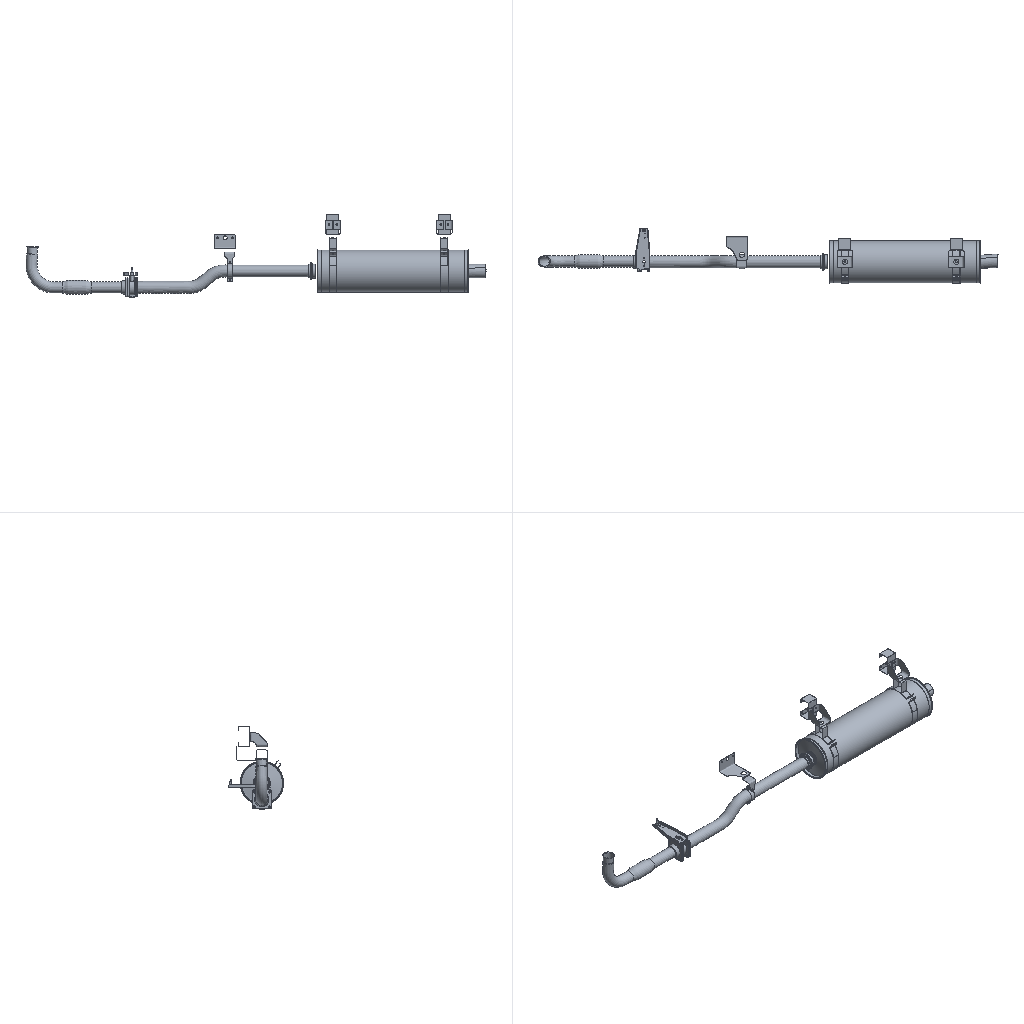Simulation study | nastran
Set-up summary:
category,name,step,type,value,unit,region
solver,nx_nastran
units,not stated in the deck,,not stated
analysis,deck,,modal,modal
analysis,solution,,SOL,103
load_step,SUBCASE 1,1,SUBCASE,SPC=None LOAD=None
mesh,nodes,,,119114
mesh,elements,,,239207
element_type,CQUAD4,,shell,54848
element_type,CTETRA,,solid,184005
element_type,CTRIA3,,shell,354
load,load commands in deck,,count,0
bc,support commands in deck,,count,0
check,setup vs results,,match,"every grid point's frame and coordinates and every element id; grid points of CQUAD4, CTETRA, CTRIA3 elements"
Nastran input file, long lists of numbers shortened:
$$------------------------------------------------------------------------------$
$$                                                                              $
$$ NASTRAN Input Deck Generated by HyperMesh Version  :10.0buil                 $
$$ Generated using HyperMesh-Nastran Template Version : 10.0build60
$$                                                                              $
$$   Template:  general                                                         $
$$                                                                              $
$$------------------------------------------------------------------------------$
$$------------------------------------------------------------------------------$
$$                      Executive Control Cards                                 $
$$------------------------------------------------------------------------------$
SOL 103
CEND
$$------------------------------------------------------------------------------$
$$                      Case Control Cards                                      $
$$------------------------------------------------------------------------------$
  DISPLACEMENT = ALL
$
$HMNAME LOADSTEP               1"modal"
SUBCASE       1
  LABEL= modal
  METHOD(STRUCTURE) =        1
$$------------------------------------------------------------------------------$
$$                      Bulk Data Cards                                         $
$$------------------------------------------------------------------------------$
BEGIN BULK
PARAM,POST,-1
$$
$$  GRID Data
$$
GRID          15        651.7036269.0462-556.3
GRID         158        651.0115268.8809-557.749
$ (119112 more lines like these left out)
$$
$$  SPOINT Data
$$
$$
$$------------------------------------------------------------------------------$
$$             Group Definitions                                                $
$$------------------------------------------------------------------------------$
$
$ RBE2 Elements - Single dependent node
$
RBE2        6841    4629  123456    3564
RBE2        6840    4628  123456    3563
$ (313 more lines like these left out)
$
$HMMOVE        8
$           6841    6840    6839    6838    6837    6836    6835    6834    6833
$           6832    6831    6830    6829    6828    6827    6826    6825    6824
$           6823    6822    6821    6820    6819    6818    6817    6816    6815
$           6814    6813    6812    6811    6810    6809    6808    6807    6806
$           6805    6804    6803    6802    6801    6800    6799    6798    6797
$           6796    6795    6794  648943THRU      648995  648997THRU      649001
$         649004THRU      649010  649012  649014  649016THRU      649020  649022
$       THRU      649024  649026THRU      649028  649033THRU      649035  649037
$         649039THRU      649040  649042THRU      649048  649050THRU      649053
$         649055THRU      649056  649058THRU      649059  649061THRU      649063
$         649065THRU      649069  649079THRU      649081  649083THRU      649090
$         649092THRU      649162  649164THRU      649190  649197THRU      649229
$         649231THRU      649248
$
$$
$$ RBE2 Elements - Multiple dependent nodes
$$
RBE2      159642   74835  123456   66951   67011   67130   67146   67147+
+          70841   70842   70843   70844   70845   70846   70847   70848+
+          70849   70850   70851   70852   70853   70854   70855   70856+
+          70857   70858   70859   70860   70861   70862   70863   70864+
+          70865   70866   70867   70868   70869   70870   70871   70872+
+          70873   70874   70875   70876   70877   70878   70879   70880+
+          70881   70882   70883   70884   70885   70886   70887   70888+
+          70889   70890   70891   70892   70893   70894   70895   70896+
+          70897   70898   70899   70900   70901   70902   70903   70904+
+          70905   70906   70907   70908   70909   70910   70911   70912+
+          70913   70914   70915   70916   70917   70918   70919   70920+
+          70921   70922   70923   70924   70925   70926   70927   70928+
+          70929   70930   70931   70932   70933   70934   70935   70936+
+          70937   70938   70939   70940   70941   70942   70943   70944+
+          70945   70946   70947   70948   70949   70950   70951   70952+
+          70953   70954   70955   70956   70957   70958   70959   70960+
+          70961   70962   70963   70964   70965   70966   70967   70968+
+          70969   70970   70971   70972   70973   70974   70975   70976+
+          70977   70978   70979   70980   70981   70982   70983   70984+
+          70985   70986   70987   70988   70989   70990   70991   70992+
+          70993   70994   70995   70996   70997   70998   70999   71000+
+          71001   71002   71003   71004   71005   71006   71007   71008+
+          71009   71010   71011   71012   71013   71014   71015   71016+
+          71017   71018   71019   71020   71021   71022   71023   71024+
+          71025   71026   71027   71028   71029   71030   71031   71032+
+          71033   71034   71035   71036   71037   71038   71039   71040+
+          71041   71042   71043   71044   71045   71046   71047   71048+
+          71049   71050   71051   71052   71053   71054   71055   71056+
+          71057   71058   71059   71060   71061   71062   71063   71064+
+          71065   71066   71067   71068   71069   71070   71071   71072+
+          71073   71074   71075   71076   71077   71078   71079   71080+
+          71081   71082   71083   71084   71085   71086   71087   71088+
+          71089   71090   71091   71092   71093   71094   71095   71096+
+          71097   71098   71099   71100   71101   71102   71103   71104+
+          71105   71106   71107   71108   71109   71110   71111   71112+
+          71113   71114   71115   71116   71117   71118   71119   71120+
+          71121   71122   71123   71124   71125   71126   71127   71128+
+          71129   71130   71131   71132   71133   71134   71135   71136+
+          71137   71138   71139   71140   71141   71142   71143   71144+
+          71145   71146   71147   71148   71149   71150   71151   71152+
+          71153   71154   71155   71156   71157   71158   71159   71160+
+          71161   71162   71163   71164   71165   71166   71167   71168+
+          71169   71170   71171   71172   71173   71174   71175   71176+
+          71177   71178   71179   71180   71181   71182   71183   71184+
+          71185   71186   71187   71188   71189   71190   71191   71192+
+          71193   71194   71195   71196   71197   71198   71199   71200+
+          71201   71202   71203   71204   71205   71206   71207   71208+
+          71209   71210   71211   71212   71213   71214   71215   71216+
+          71217   71218   71219   71220   71221   71222   71223   71224+
+          71225   71226   71227   71228   71229   71230   71231   71232+
+          71233   71234   71235   71236   71237   71238   71239   71240+
+          71241   71242   71243   71244   71245   71246   71247   71248+
+          71249   71250   71251   71252   71253   71254   71255   71256+
+          71257   71258   71259   71260   71261   71262   71263   71264+
+          71265   71266   71267   71268   71269   71270   71271   71272+
+          71273   71274   71275   71276   71277   71278   71279   71280+
+          71281   71282   71283   71284   71285   71286   71287   71288+
+          71289   71290   71291   71292   71293   71294   71295   71296+
+          71297   71298   71299   71300   71301   71302   71303   71304+
+          71305   71306   71307   71308   71309   71310   71311   71312+
+          71313   71314   71315   71316   71317   71318   71319   71320+
+          71321   71322   71323   71324   71325   71326   71327   71328+
+          71329   71330   71331   71332   71333   71334   71335   71336+
+          71337   71338   71339   71340   71341   71342   71343   71344+
+          71345   71346   71347   71348   71349   71350   71351   71352+
+          71353   71354   71355   71356   71357   71358   71359   71360+
+          71361   71362   71363   71364   71365   71366   71367   71368+
+          71369   71370   71371   71372   71373   71374   71375   71376+
+          71377   71378   71379   71380   71381   71382   71383   71384+
+          71385   71386   71387   71388   71389   71390   71391   71392+
+          71393   71394   71395   71396   71397   71398   71399   71400+
+          71401   71402   71403   71404   71405   71406   71407   71408+
+          71409   71410   71411   71412   71413   71414   71415   71416+
+          71417   71418   71419   71420   71421   71422   71423   71424+
+          71425   71426   71427   71428   71429   71430   71431   71432+
+          71433   71434   71435   71436   71437   71438   71439   71440+
+          71441   71442   71443   71444   71445   71446   71447   71448+
+          71449   71450   71451   71452   71453   71454   71455   71456+
+          71457   71458   71459   71460   71461   71462   71463   71464+
+          71465   71466   71467   71468   71469   71470   71471   71472+
+          71473   71474   71475   71476   71477   71478   71479   71480+
+          71481   71482   71483   71484   71485   71486   71487   71488+
+          71489   71490   71491   71492   71493   71494   71495   71496+
+          71497   71498   71499   71500   71501   71502   71503   71504+
+          71505   71506   71507   71508   71509   71510   71511   71512+
+          71513   71514   71515   71516   71517   71518   71519   71520+
+          71521   71522   71523   71524   71525   71526   71527   71528+
+          71529   71530   71531   71532   71533   71534   71535   71536+
+          71537   71538   71539   71540   71541   71542   71543   71544+
+          71545   71546   71547   71548   71549   71550   71551   71552+
+          71553   71554   71555   71556   71557   71558   71559   71560+
+          71561   71562   71563   71564   71565   71566   71567   71568+
+          71569   71570   71571   71572   71573   71574   71575   71576+
+          71577   71578   71579   71580   71581   71582   71583   71584+
+          71585   71586   71587   71588   71589   71590   71591   71592+
+          71593   71594   71595   71596   71597   71598   71599   71600+
+          71601   71602   71603   71604   71605   71606   71607   71608+
+          71609   71610   71611   71612   71613   71614   71615   71616+
+          71617   71618   71619   71620   71621   71622   71623   71624+
+          71625   71626   71627   71628   71629   71630   71631   71632+
+          71633   71634   71635   71636   71637   71638   71639   71640+
+          71641   71642   71643   71644   71645   71646   71647   71648+
+          71649   71650   71651   71652   71653   71654   71655   71656+
+          71657   71658   71659   71660   71661   71662   71663   71664+
+          71665   71666   71667   71668   71669   71670   71671   71672+
+          71673   71674   71675   71676   71677   71678   71679   71680+
+          71681   71682   71683   71684   71685   71686   71687   71688+
+          71689   71690   71691   71692   71693   71694   71695   71696+
+          71697   71698   71699   71700   71701   71702   71703   71704+
+          71705   71706   71707   71708   71709   71710   71711   71712+
+          71713   71714   71715   71716   71717   71718   71719   71720+
+          71721   71722   71723   71724   71725   71726   71727   71728+
+          71729   71730   71731   71732   71733   71734   71735   71736+
+          71737   71738   71739   71740   71741   71742   71743   71744+
+          71745   71746   71747   71748   71749   71750   71751   71752+
+          71753   71754   71755   71756   71757   71758   71759   71760+
+          71761   71762   71763   71764   71765   71766   71767   71768+
+          71769   71770   71771   71772   71773   71774   71775   71776+
+          71777   71778   71779   71780   71781   71782   71783   71784+
+          71785   71786   71787   71788   71789   71790   71791   71792+
+          71793   71794   71795   71796   71797   71891   71892   71893+
+          71894   71895   71896   71897   71898   71899   71900   71901+
+          71902   71903   71904   71905   71906   71907   71908   71909+
+          71910   71911   71912   71913   71914   71915   71916   71917+
+          71918   71919   71920   71921   71922   71923   71924   71925+
+          71926   71927   71928   71929   71930   71931   71932   71933+
+          71934   71935   71936   71937   71938   71939   71940   71941+
+          71942   71943   71944   71945   71946   71947   71948   71949+
+          71950   71951   71952   71953   71954   71955   71956   71957+
+          71958   71959   71960   71961   71962   71963   71964   71965+
+          71966   71967   71968   71969   71970   71971   71972   71973+
+          71974   71975   71976   71977   71978   71979   71980   71981+
+          71982   71983   71984   71985   71986   71987   71988   71989+
+          71990   71991
RBE2      166925   74836  123456   58298   58299   58302   58303   58306+
+          58307   58310   58311   58314   58315   58318   58319   58322+
+          58323   58326   58327   58330   58331   58334   58335   58338+
+          58339   58342   58343   58346   58347   67796   69549   69550+
+          69551   69552   69553   69554   69555   69556   69557   69558+
+          69559   69560   69561   69562   69563   69564   69565   69566+
+          69567   69568   69569   69570   69571   69572   69573   69574+
+          69575   69576   69577   69578   69579   69580   69581   69582+
+          69583   69584   69585   69586   69587   69588   69589   69590+
+          69591   69592   69593   69594   69595   69596   69597   69598+
+          69599   69600   69601   69602   69603   69604   69605   69606+
+          69607   69608   69609   69610   69611   69612   69613   69614+
+          69615   69616   69617   69618   69619   69620   69621   69622+
+          69623   69624   69625   69626   69627   69628   69629   69630+
+          69631   69632   69633   69634   69635   69636   69637   69638+
+          69639   69640   74636   74637   74638   74639   74640   74641+
+          74642   74643   74644   74645   74646   74647   74648   74649+
+          74650   74651   74652   74653   74654   74655   74656   74657+
+          74658   74659   74660   74661   74662   74663   74664   74665+
+          74666   74667   74668   74669   74670   74671   74672   74673+
+          74674   74675   74676   74677   74678   74679   74680   74681+
+          74682   74683   74684   74685   74686   74687   74688   74689+
+          74690   74691   74692   74693   74694   74695   74696   74697+
+          74698   74699   74700   74701   74702   74703   74704   74705+
+          74706   74707   74708   74709   74710   74711   74712   74713+
+          74714   74715   74716   74717   74718   74719   74720   74721+
+          74722   74723   74724   74725   74726   74727   74728   74729+
+          74730   74731   74732   74733   74734   74735   74736   74737+
+          74738   74739   74740   74741   74742   74743   74744   74745+
+          74746   74747   74748   74749   74750   74751   74752   74753+
+          74754   74755   74756   74757   74758   74759   74760   74761+
+          74762   74763   74764   74765   74766   74767   74768   74769+
+          74770   74771   74772   74773   74774   74775   74776   74777+
+          74778   74779   74780   74781   74782   74783   74784   74785+
+          74786   74787   74788   74789   74790   74791   74792   74793+
+          74794   74795   74796   74797   74798   74799   74800   74801+
+          74802   74803   74804   74805   74806   74807   74808   74809+
+          74810   74811   74812   74813   74814   74815   74816   74817+
+          74818   74819   74820   74821
$ (2087 more lines like these left out)
$
$HMMOVE        8
$         159642  166925  643640THRU      643641  648884THRU      648896  648898
$       THRU      648903  648905THRU      648931  648933THRU      648942  649070
$       THRU      649077  649191THRU      649196  649249THRU      649254  649256
$       THRU      649265  649269  649267THRU      649268  649266  649270THRU
$         649280  649282THRU      649322
$
$$
$$  CTRIA3 Data
$$
CTRIA3      6301       1    5904    5931    5881
CTRIA3      6297       1    5882    5937    5888
$ (352 more lines like these left out)
$
$HMMOVE        4
$           6301    6297    6286    6267    6240    6209    6155    6136    5285
$           6031    6020    6014    5901    5776    5373    5404    5466    5651
$ (65 more lines like these left out)
CQUAD4      5256       1     207     208    4900    4909
CQUAD4      5255       1    4896    4898    4903    4899
$ (54846 more lines like these left out)
$
$HMMOVE        4
$           5256    5255    6327    6326    6325    6324    6323    6322    6321
$           6320    6319    6318    5275    5272    5270    6317    6316    6315
$ (469 more lines like these left out)
CTETRA     43726       8   14044   14046   14040   13409
CTETRA     43725       8   13409   13375   14040   13426
$ (184003 more lines like these left out)
$
$HMMOVE        9
$          43726   43725   43724   43723   43722   43721   43720   43719   43718
$          43717   43716   43715   43714   43713   43712   43711   43710   43709
$ (746 more lines like these left out)
PSHELL         1       11.5            1               1
$
$HMNAME PROP                   2"550" 4
$HWCOLOR PROP                  2      11
PSHELL         2       15.5            1               1
$
$HMNAME PROP                   3"400" 4
$HWCOLOR PROP                  3      11
PSHELL         3       14.0            1               1
$
$HMNAME PROP                   4"600" 4
$HWCOLOR PROP                  4      11
PSHELL         4       16.0            1               1
$
$HMNAME PROP                   5"500" 4
$HWCOLOR PROP                  5      11
PSHELL         5       15.0            1               1
$
$HMNAME PROP                   6"160" 4
$HWCOLOR PROP                  6      11
PSHELL         6       11.6            1               1
$
$HMNAME PROP                   7"120" 4
$HWCOLOR PROP                  7      11
PSHELL         7       11.2            1               1
$$
$$  PSOLID Data
$
$HMNAME PROP                   8"solid" 5
$HWCOLOR PROP                  8      11
PSOLID         8       1
$$
$$------------------------------------------------------------------------------$
$$                      Material Definition Cards                               $
$$------------------------------------------------------------------------------$
$$--------------------------------------------------------------
$$ HYPERMESH TAGS
$$--------------------------------------------------------------
$$BEGIN TAGS
$$END TAGS
$$
$$  MAT1 Data
$
$HMNAME MAT                    1"steel" "MAT1"
$HWCOLOR MAT                   1      11
MAT1           1210000.0        0.3     7.85E-09
$$
$$
$$
$$------------------------------------------------------------------------------$
$ (31 more lines like these left out)
EIGRL          10.0                   16                            MASS
$
ENDDATA
Results summary:
result,analysis,,,modal
result,primary field,,,eigenvectors